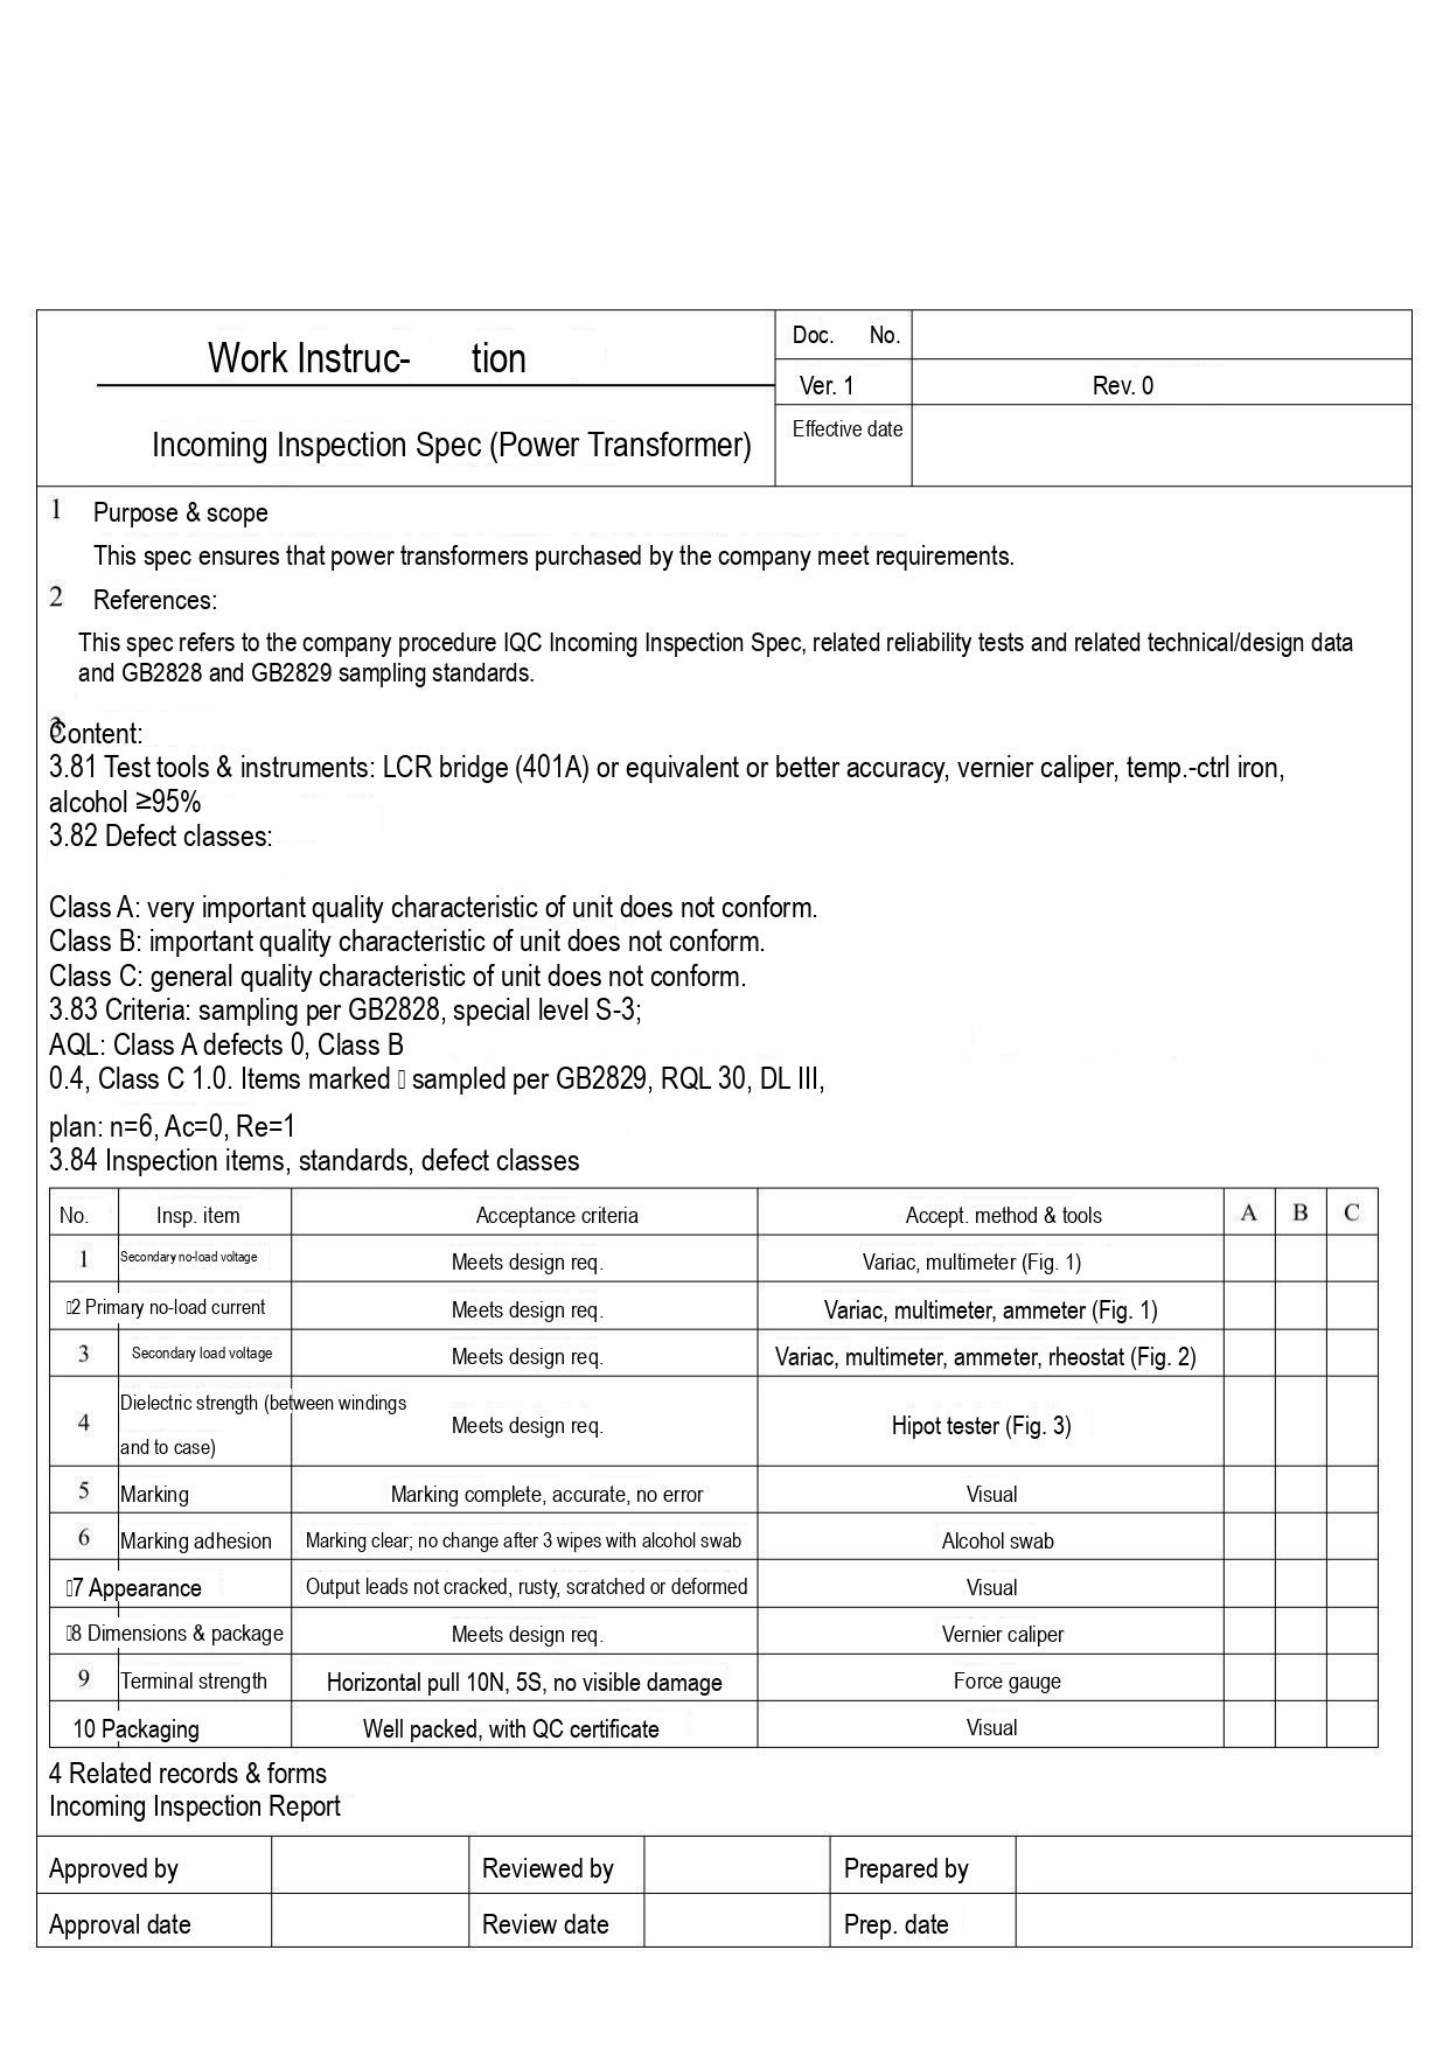| Work Instruc- tion<br>Incoming Inspection Spec (Power Transformer) | Doc. No. | |
|---|---|---|
| | Ver. 1 | Rev. 0 |
| | Effective date | |

1 Purpose & scope

This spec ensures that power transformers purchased by the company meet requirements.

2 References:

This spec refers to the company procedure IQC Incoming Inspection Spec, related reliability tests and related technical/design data and GB2828 and GB2829 sampling standards.

3 Content:
3.81 Test tools & instruments: LCR bridge (401A) or equivalent or better accuracy, vernier caliper, temp.-ctrl iron, alcohol ≥95%
3.82 Defect classes:

Class A: very important quality characteristic of unit does not conform.
Class B: important quality characteristic of unit does not conform.
Class C: general quality characteristic of unit does not conform.
3.83 Criteria: sampling per GB2828, special level S-3;
AQL: Class A defects 0, Class B
0.4, Class C 1.0. Items marked ▯ sampled per GB2829, RQL 30, DL III,

plan: n=6, Ac=0, Re=1
3.84 Inspection items, standards, defect classes

| No. | Insp. item | Acceptance criteria | Accept. method & tools | A | B | C |
|---|---|---|---|---|---|---|
| 1 | Secondary no-load voltage | Meets design req. | Variac, multimeter (Fig. 1) | | | |
| ▯2 | Primary no-load current | Meets design req. | Variac, multimeter, ammeter (Fig. 1) | | | |
| 3 | Secondary load voltage | Meets design req. | Variac, multimeter, ammeter, rheostat (Fig. 2) | | | |
| 4 | Dielectric strength (between windings and to case) | Meets design req. | Hipot tester (Fig. 3) | | | |
| 5 | Marking | Marking complete, accurate, no error | Visual | | | |
| 6 | Marking adhesion | Marking clear; no change after 3 wipes with alcohol swab | Alcohol swab | | | |
| ▯7 | Appearance | Output leads not cracked, rusty, scratched or deformed | Visual | | | |
| ▯8 | Dimensions & package | Meets design req. | Vernier caliper | | | |
| 9 | Terminal strength | Horizontal pull 10N, 5S, no visible damage | Force gauge | | | |
| 10 | Packaging | Well packed, with QC certificate | Visual | | | |

4 Related records & forms
Incoming Inspection Report

| Approved by | | Reviewed by | | Prepared by | |
|---|---|---|---|---|---|
| Approval date | | Review date | | Prep. date | |
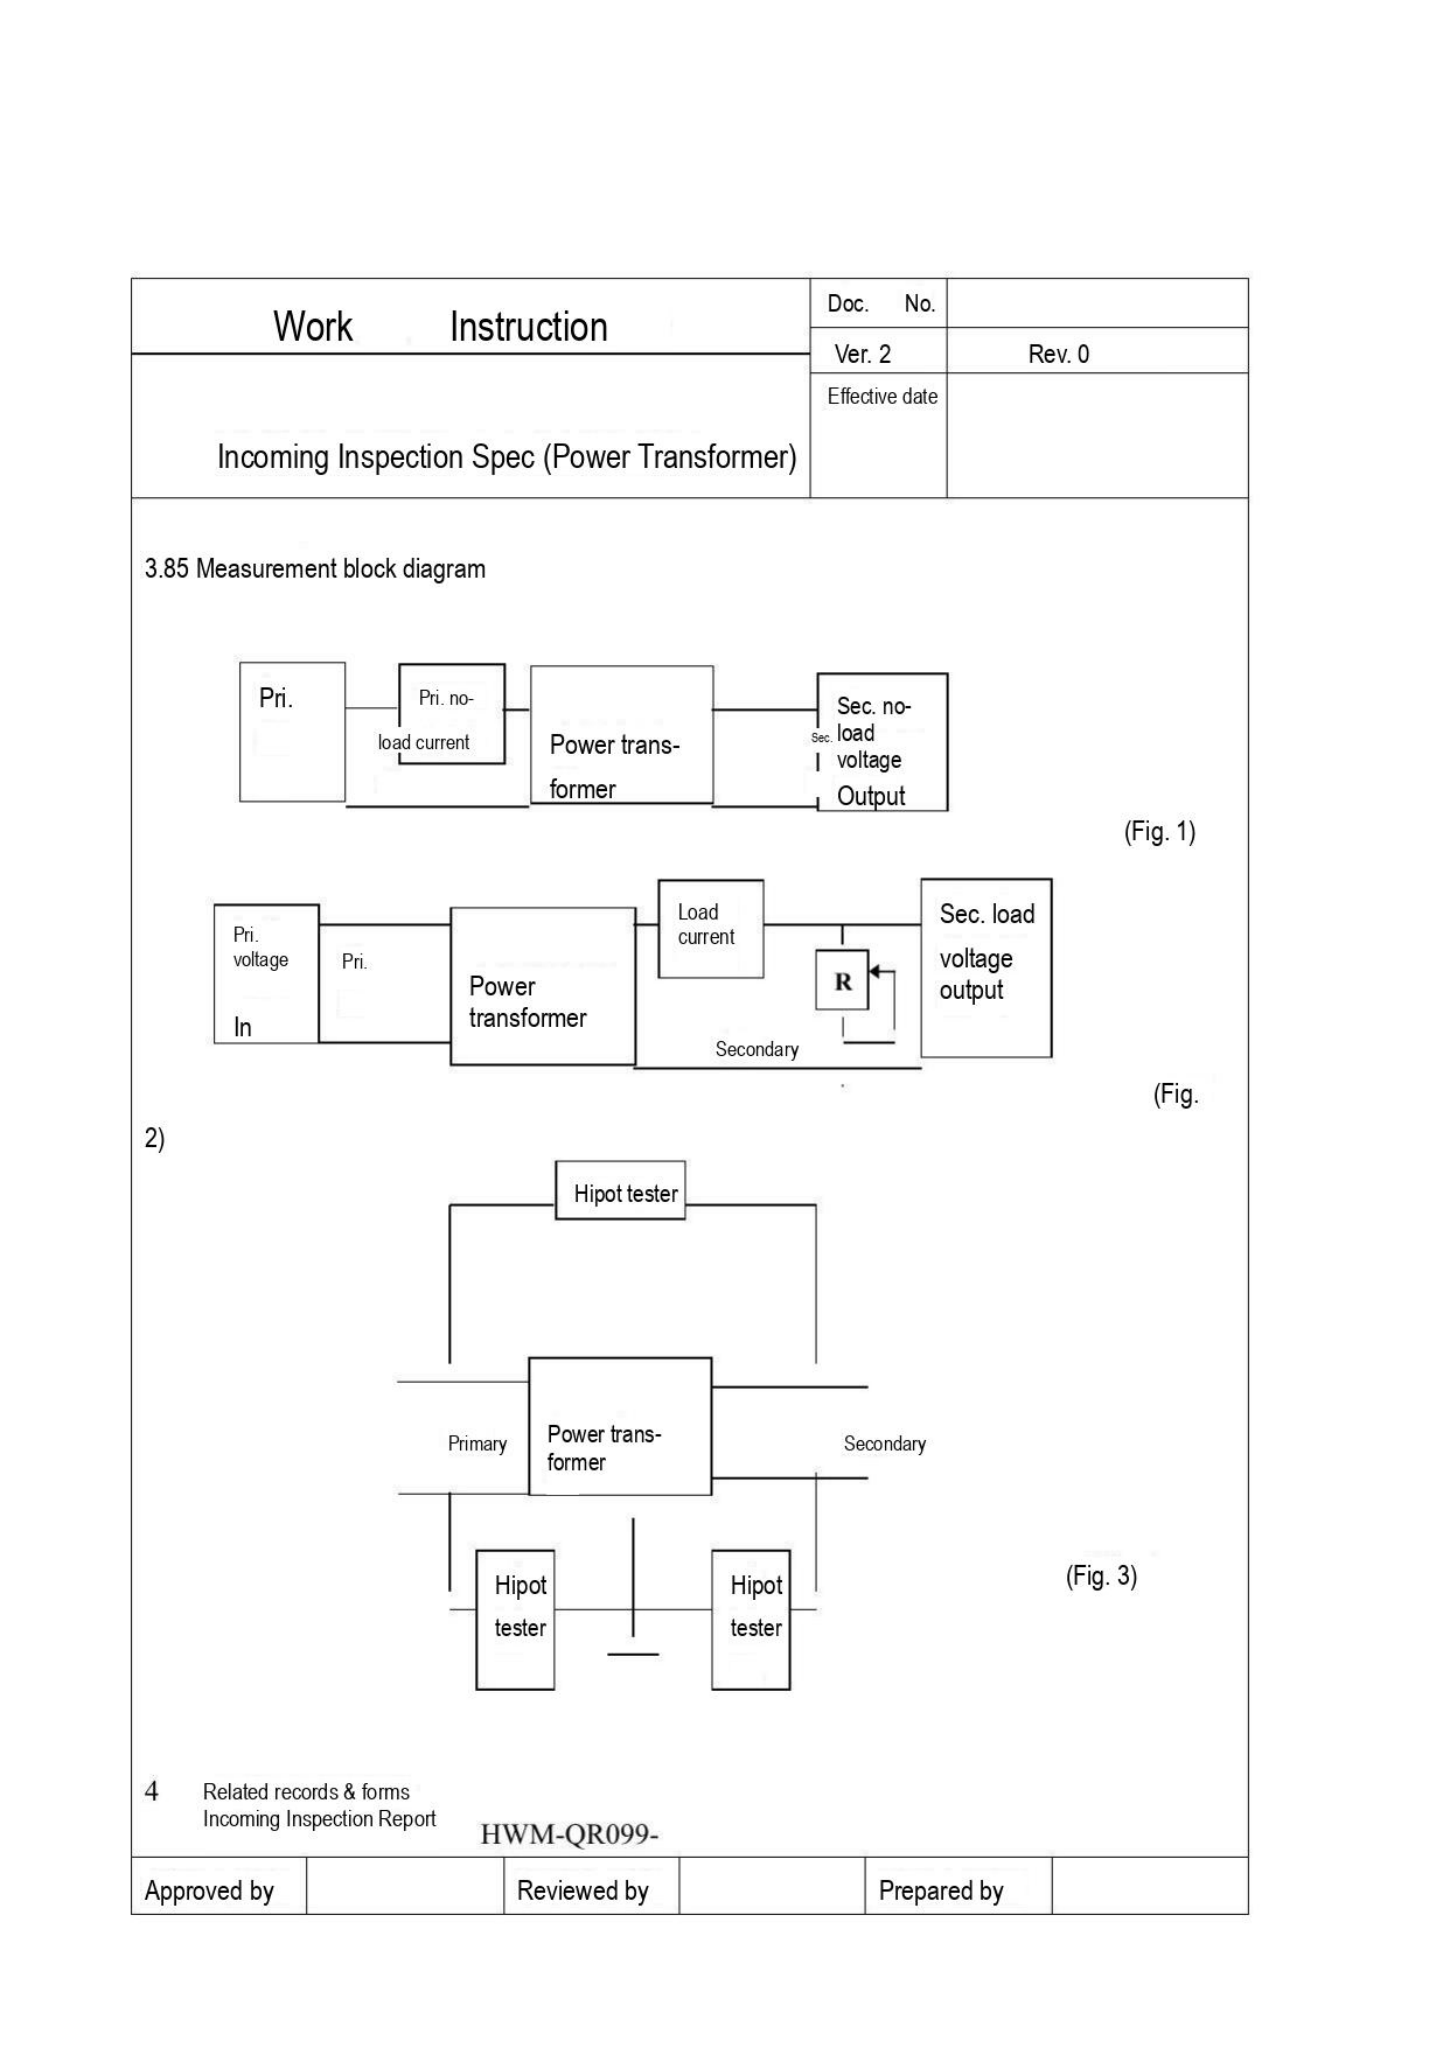| Work Instruction | Doc. No. | |
|---|---|---|
| | Ver. 2 | Rev. 0 |
| Incoming Inspection Spec (Power Transformer) | Effective date | |

3.85 Measurement block diagram

Pri.

Pri. no-load current

Power trans-former

Sec.

Sec. no-load voltage Output

(Fig. 1)

Pri. voltage In

Pri.

Power transformer

Load current

R

Secondary

Sec. load voltage output

(Fig. 2)

Hipot tester

Primary

Power trans-former

Secondary

Hipot tester

Hipot tester

(Fig. 3)

4 Related records & forms
Incoming Inspection Report HWM-QR099-

| Approved by | | Reviewed by | | Prepared by | |
|---|---|---|---|---|---|
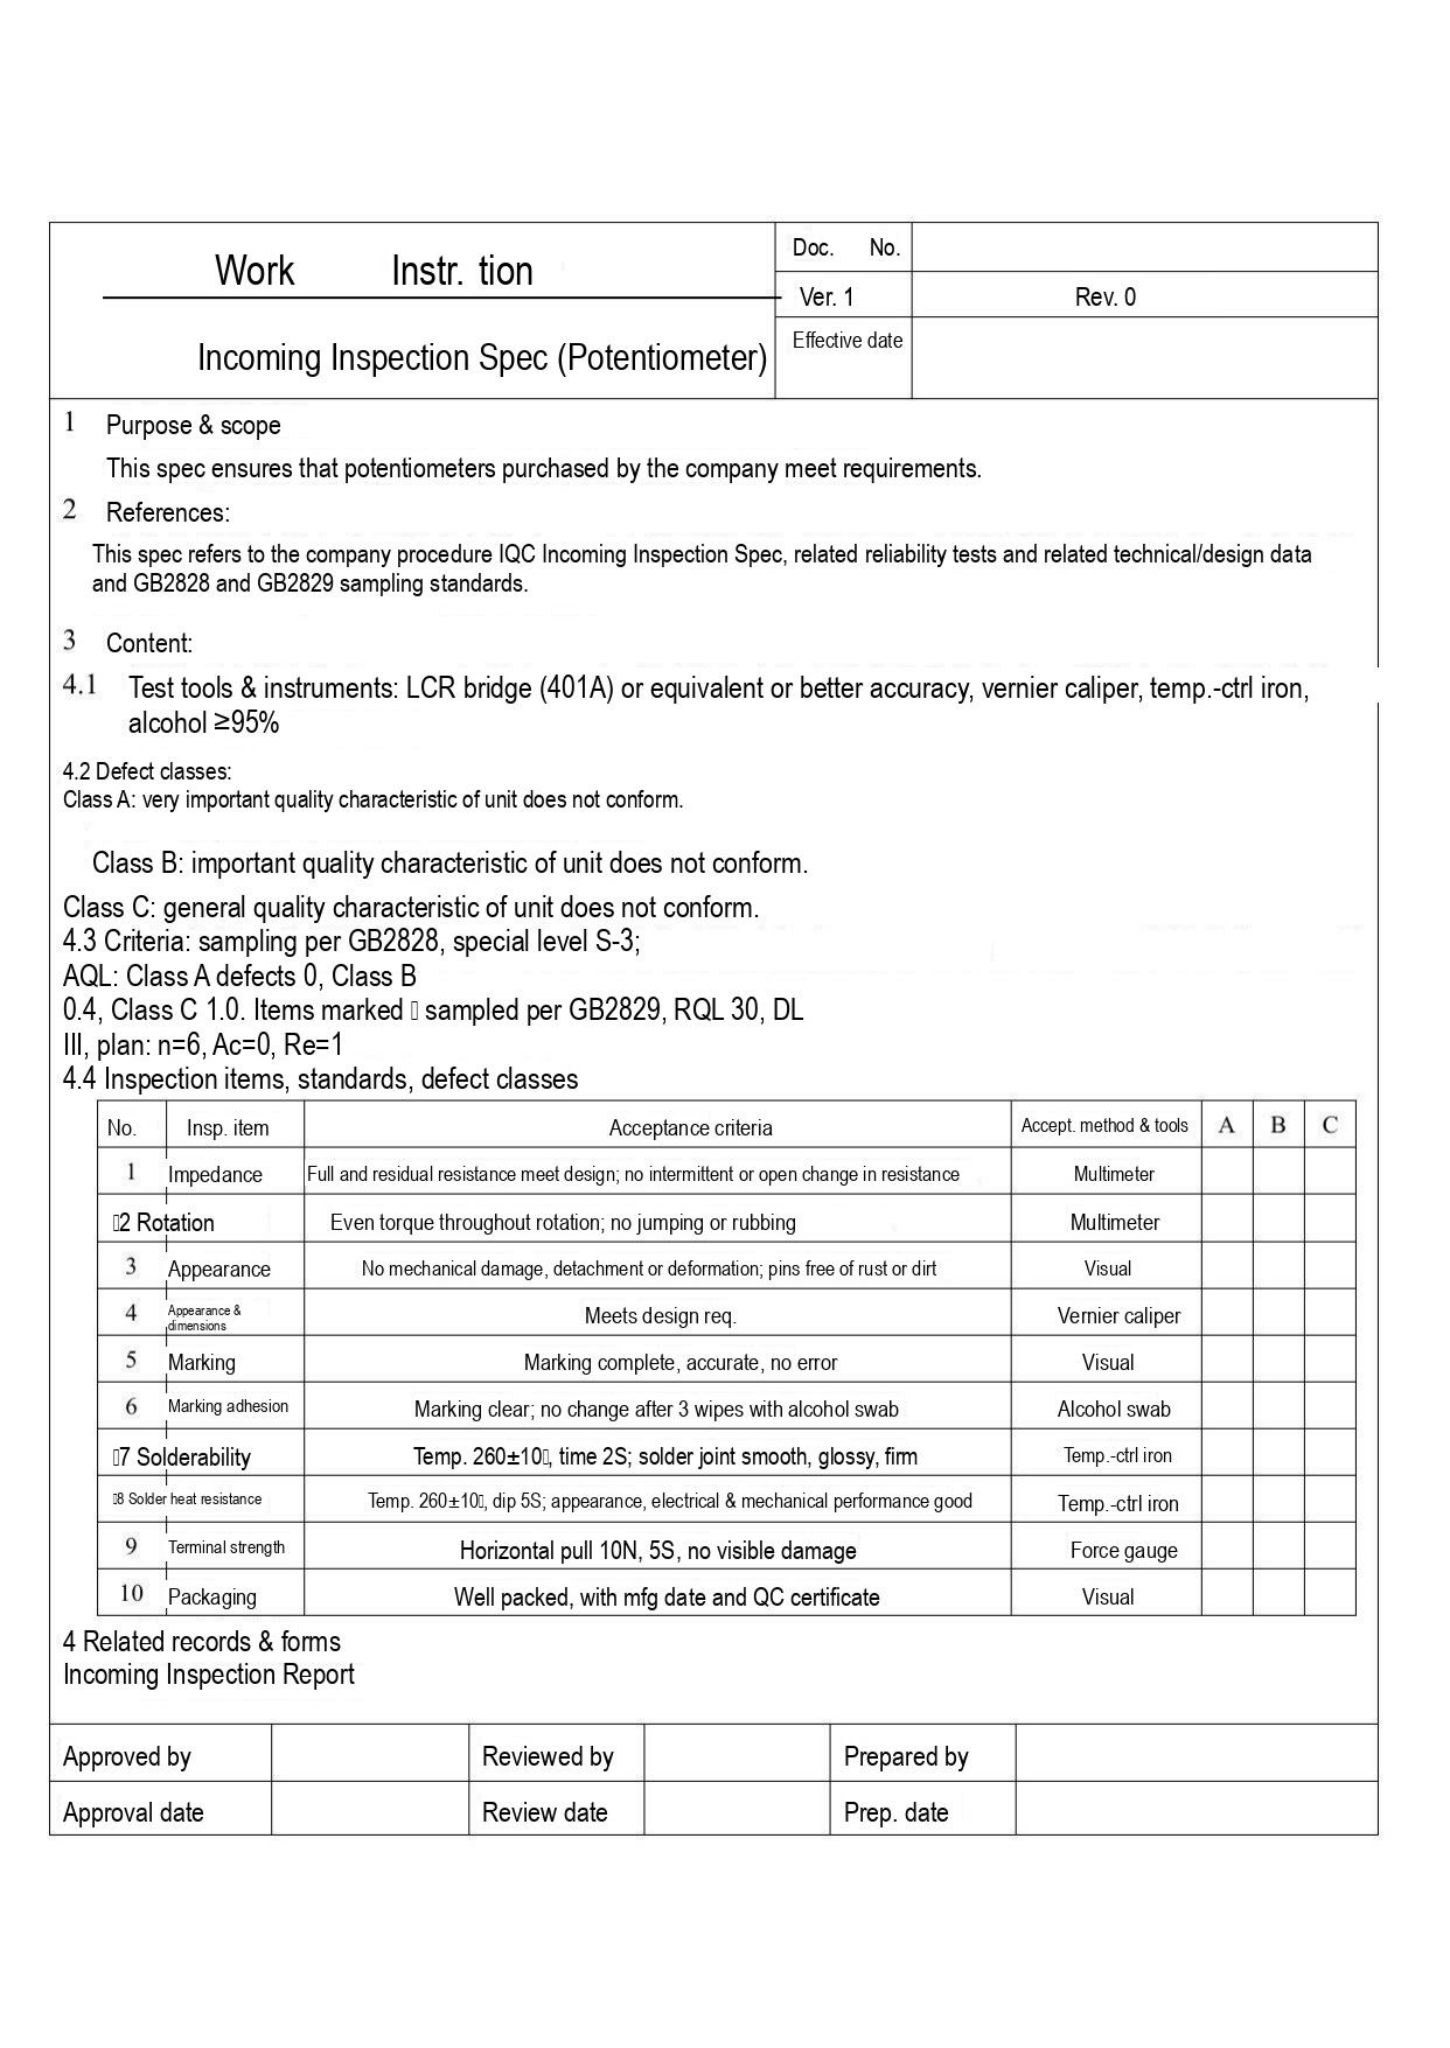| Work Instr. tion<br>Incoming Inspection Spec (Potentiometer) | Doc. No. | |
|---|---|---|
| | Ver. 1 | Rev. 0 |
| | Effective date | |

1 Purpose & scope

This spec ensures that potentiometers purchased by the company meet requirements.

2 References:

This spec refers to the company procedure IQC Incoming Inspection Spec, related reliability tests and related technical/design data and GB2828 and GB2829 sampling standards.

3 Content:

4.1 Test tools & instruments: LCR bridge (401A) or equivalent or better accuracy, vernier caliper, temp.-ctrl iron, alcohol ≥95%

4.2 Defect classes:
Class A: very important quality characteristic of unit does not conform.

Class B: important quality characteristic of unit does not conform.

Class C: general quality characteristic of unit does not conform.
4.3 Criteria: sampling per GB2828, special level S-3;
AQL: Class A defects 0, Class B
0.4, Class C 1.0. Items marked sampled per GB2829, RQL 30, DL
III, plan: n=6, Ac=0, Re=1
4.4 Inspection items, standards, defect classes

| No. | Insp. item | Acceptance criteria | Accept. method & tools | A | B | C |
|---|---|---|---|---|---|---|
| 1 | Impedance | Full and residual resistance meet design; no intermittent or open change in resistance | Multimeter | | | |
| 2 | Rotation | Even torque throughout rotation; no jumping or rubbing | Multimeter | | | |
| 3 | Appearance | No mechanical damage, detachment or deformation; pins free of rust or dirt | Visual | | | |
| 4 | Appearance & dimensions | Meets design req. | Vernier caliper | | | |
| 5 | Marking | Marking complete, accurate, no error | Visual | | | |
| 6 | Marking adhesion | Marking clear; no change after 3 wipes with alcohol swab | Alcohol swab | | | |
| 7 | Solderability | Temp. 260±10, time 2S; solder joint smooth, glossy, firm | Temp.-ctrl iron | | | |
| 8 | Solder heat resistance | Temp. 260±10, dip 5S; appearance, electrical & mechanical performance good | Temp.-ctrl iron | | | |
| 9 | Terminal strength | Horizontal pull 10N, 5S, no visible damage | Force gauge | | | |
| 10 | Packaging | Well packed, with mfg date and QC certificate | Visual | | | |

4 Related records & forms
Incoming Inspection Report

| Approved by | | Reviewed by | | Prepared by | |
|---|---|---|---|---|---|
| Approval date | | Review date | | Prep. date | |
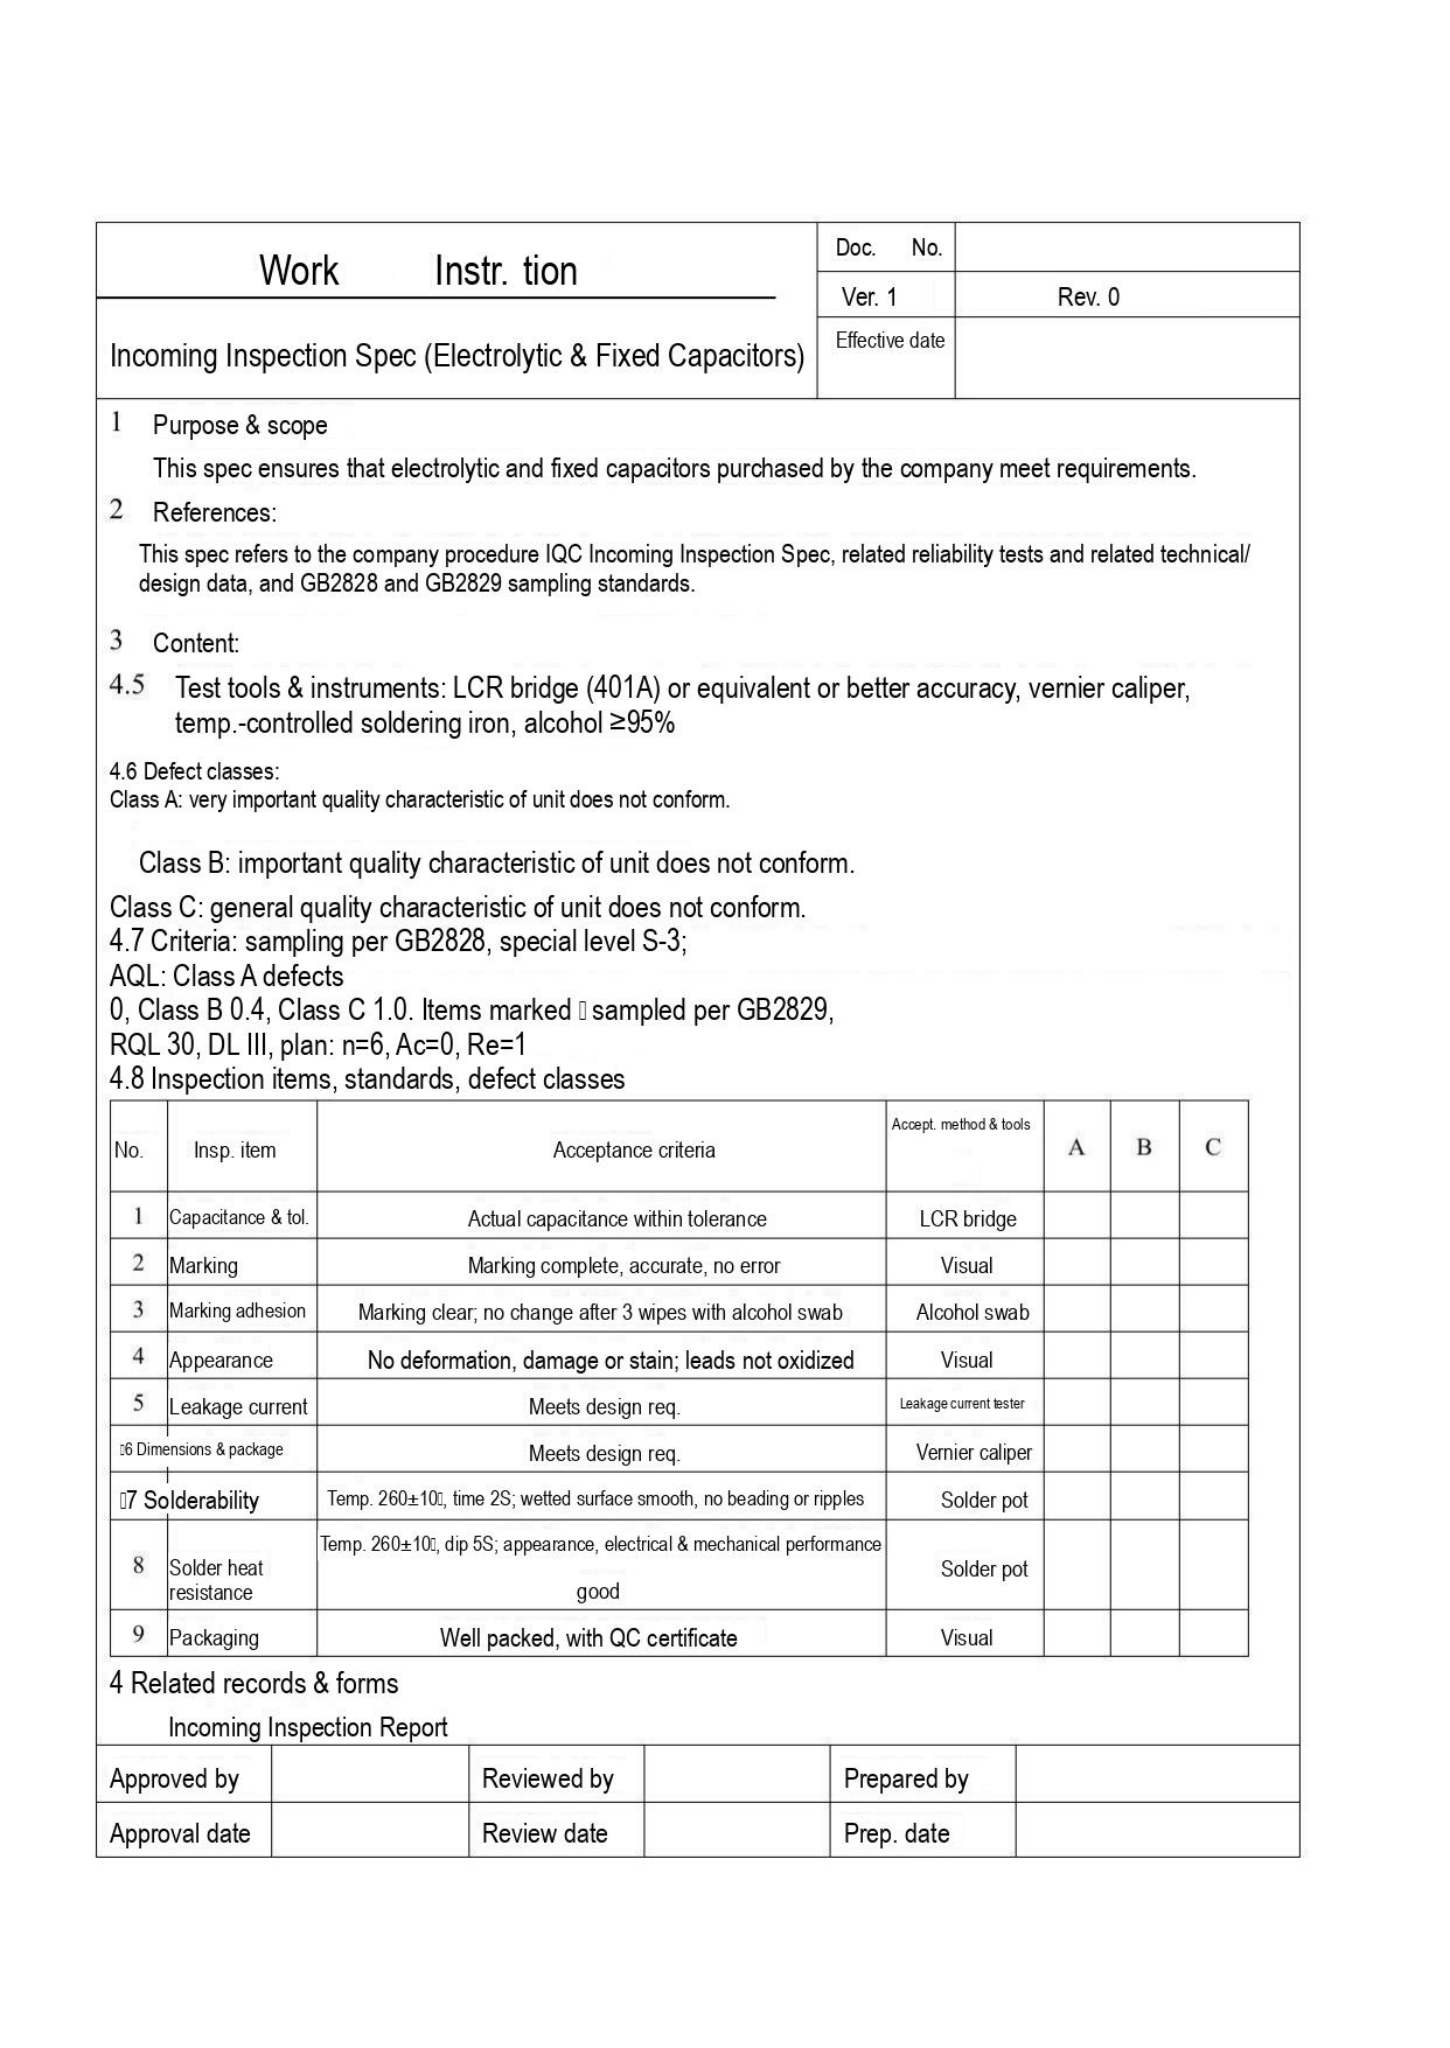| Work Instr. tion | Doc. No. | |
|---|---|---|
| | Ver. 1 | Rev. 0 |
| Incoming Inspection Spec (Electrolytic & Fixed Capacitors) | Effective date | |

1 Purpose & scope

This spec ensures that electrolytic and fixed capacitors purchased by the company meet requirements.

2 References:

This spec refers to the company procedure IQC Incoming Inspection Spec, related reliability tests and related technical/ design data, and GB2828 and GB2829 sampling standards.

3 Content:

4.5 Test tools & instruments: LCR bridge (401A) or equivalent or better accuracy, vernier caliper, temp.-controlled soldering iron, alcohol ≥95%

4.6 Defect classes:
Class A: very important quality characteristic of unit does not conform.

Class B: important quality characteristic of unit does not conform.

Class C: general quality characteristic of unit does not conform.
4.7 Criteria: sampling per GB2828, special level S-3;
AQL: Class A defects
0, Class B 0.4, Class C 1.0. Items marked sampled per GB2829,
RQL 30, DL III, plan: n=6, Ac=0, Re=1
4.8 Inspection items, standards, defect classes

| No. | Insp. item | Acceptance criteria | Accept. method & tools | A | B | C |
|---|---|---|---|---|---|---|
| 1 | Capacitance & tol. | Actual capacitance within tolerance | LCR bridge | | | |
| 2 | Marking | Marking complete, accurate, no error | Visual | | | |
| 3 | Marking adhesion | Marking clear; no change after 3 wipes with alcohol swab | Alcohol swab | | | |
| 4 | Appearance | No deformation, damage or stain; leads not oxidized | Visual | | | |
| 5 | Leakage current | Meets design req. | Leakage current tester | | | |
| 6 | Dimensions & package | Meets design req. | Vernier caliper | | | |
| 7 | Solderability | Temp. 260±10, time 2S; wetted surface smooth, no beading or ripples | Solder pot | | | |
| 8 | Solder heat resistance | Temp. 260±10, dip 5S; appearance, electrical & mechanical performance good | Solder pot | | | |
| 9 | Packaging | Well packed, with QC certificate | Visual | | | |

4 Related records & forms

Incoming Inspection Report

| Approved by | | Reviewed by | | Prepared by | |
|---|---|---|---|---|---|
| Approval date | | Review date | | Prep. date | |
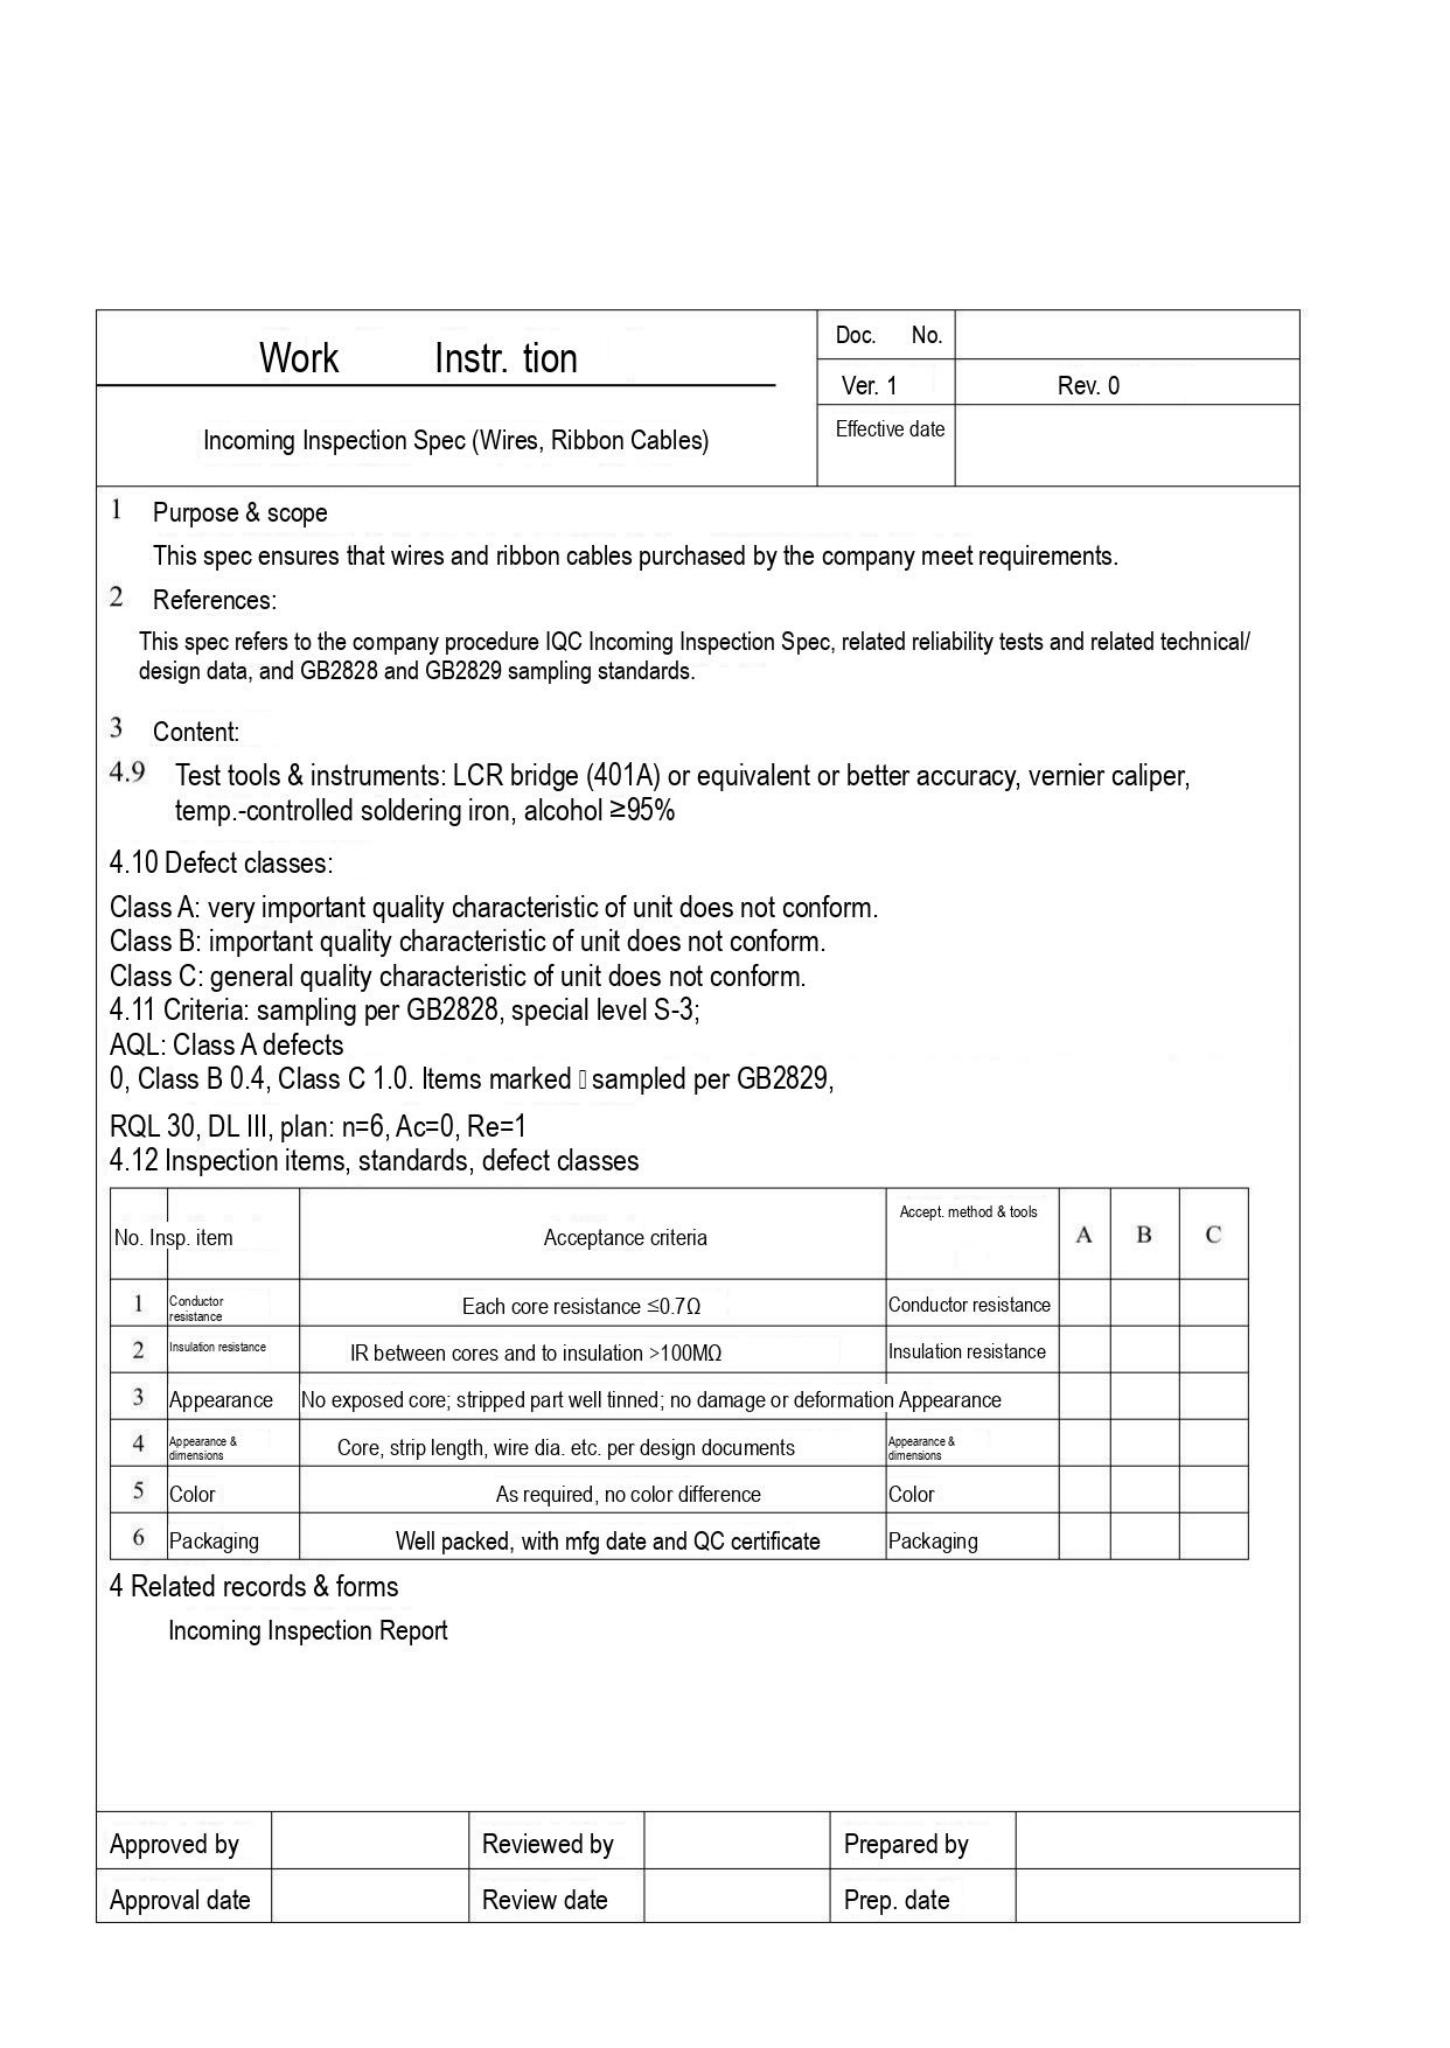| Work Instr. tion | Doc. No. | |
|---|---|---|
| | Ver. 1 | Rev. 0 |
| Incoming Inspection Spec (Wires, Ribbon Cables) | Effective date | |

1 Purpose & scope

This spec ensures that wires and ribbon cables purchased by the company meet requirements.

2 References:

This spec refers to the company procedure IQC Incoming Inspection Spec, related reliability tests and related technical/ design data, and GB2828 and GB2829 sampling standards.

3 Content:

4.9 Test tools & instruments: LCR bridge (401A) or equivalent or better accuracy, vernier caliper, temp.-controlled soldering iron, alcohol ≥95%

4.10 Defect classes:

Class A: very important quality characteristic of unit does not conform.
Class B: important quality characteristic of unit does not conform.
Class C: general quality characteristic of unit does not conform.
4.11 Criteria: sampling per GB2828, special level S-3;
AQL: Class A defects
0, Class B 0.4, Class C 1.0. Items marked sampled per GB2829,

RQL 30, DL III, plan: n=6, Ac=0, Re=1
4.12 Inspection items, standards, defect classes

| No. | Insp. item | Acceptance criteria | Accept. method & tools | A | B | C |
|---|---|---|---|---|---|---|
| 1 | Conductor resistance | Each core resistance ≤0.7Ω | Conductor resistance | | | |
| 2 | Insulation resistance | IR between cores and to insulation >100MΩ | Insulation resistance | | | |
| 3 | Appearance | No exposed core; stripped part well tinned; no damage or deformation | Appearance | | | |
| 4 | Appearance & dimensions | Core, strip length, wire dia. etc. per design documents | Appearance & dimensions | | | |
| 5 | Color | As required, no color difference | Color | | | |
| 6 | Packaging | Well packed, with mfg date and QC certificate | Packaging | | | |

4 Related records & forms

Incoming Inspection Report

| Approved by | | Reviewed by | | Prepared by | |
|---|---|---|---|---|---|
| Approval date | | Review date | | Prep. date | |
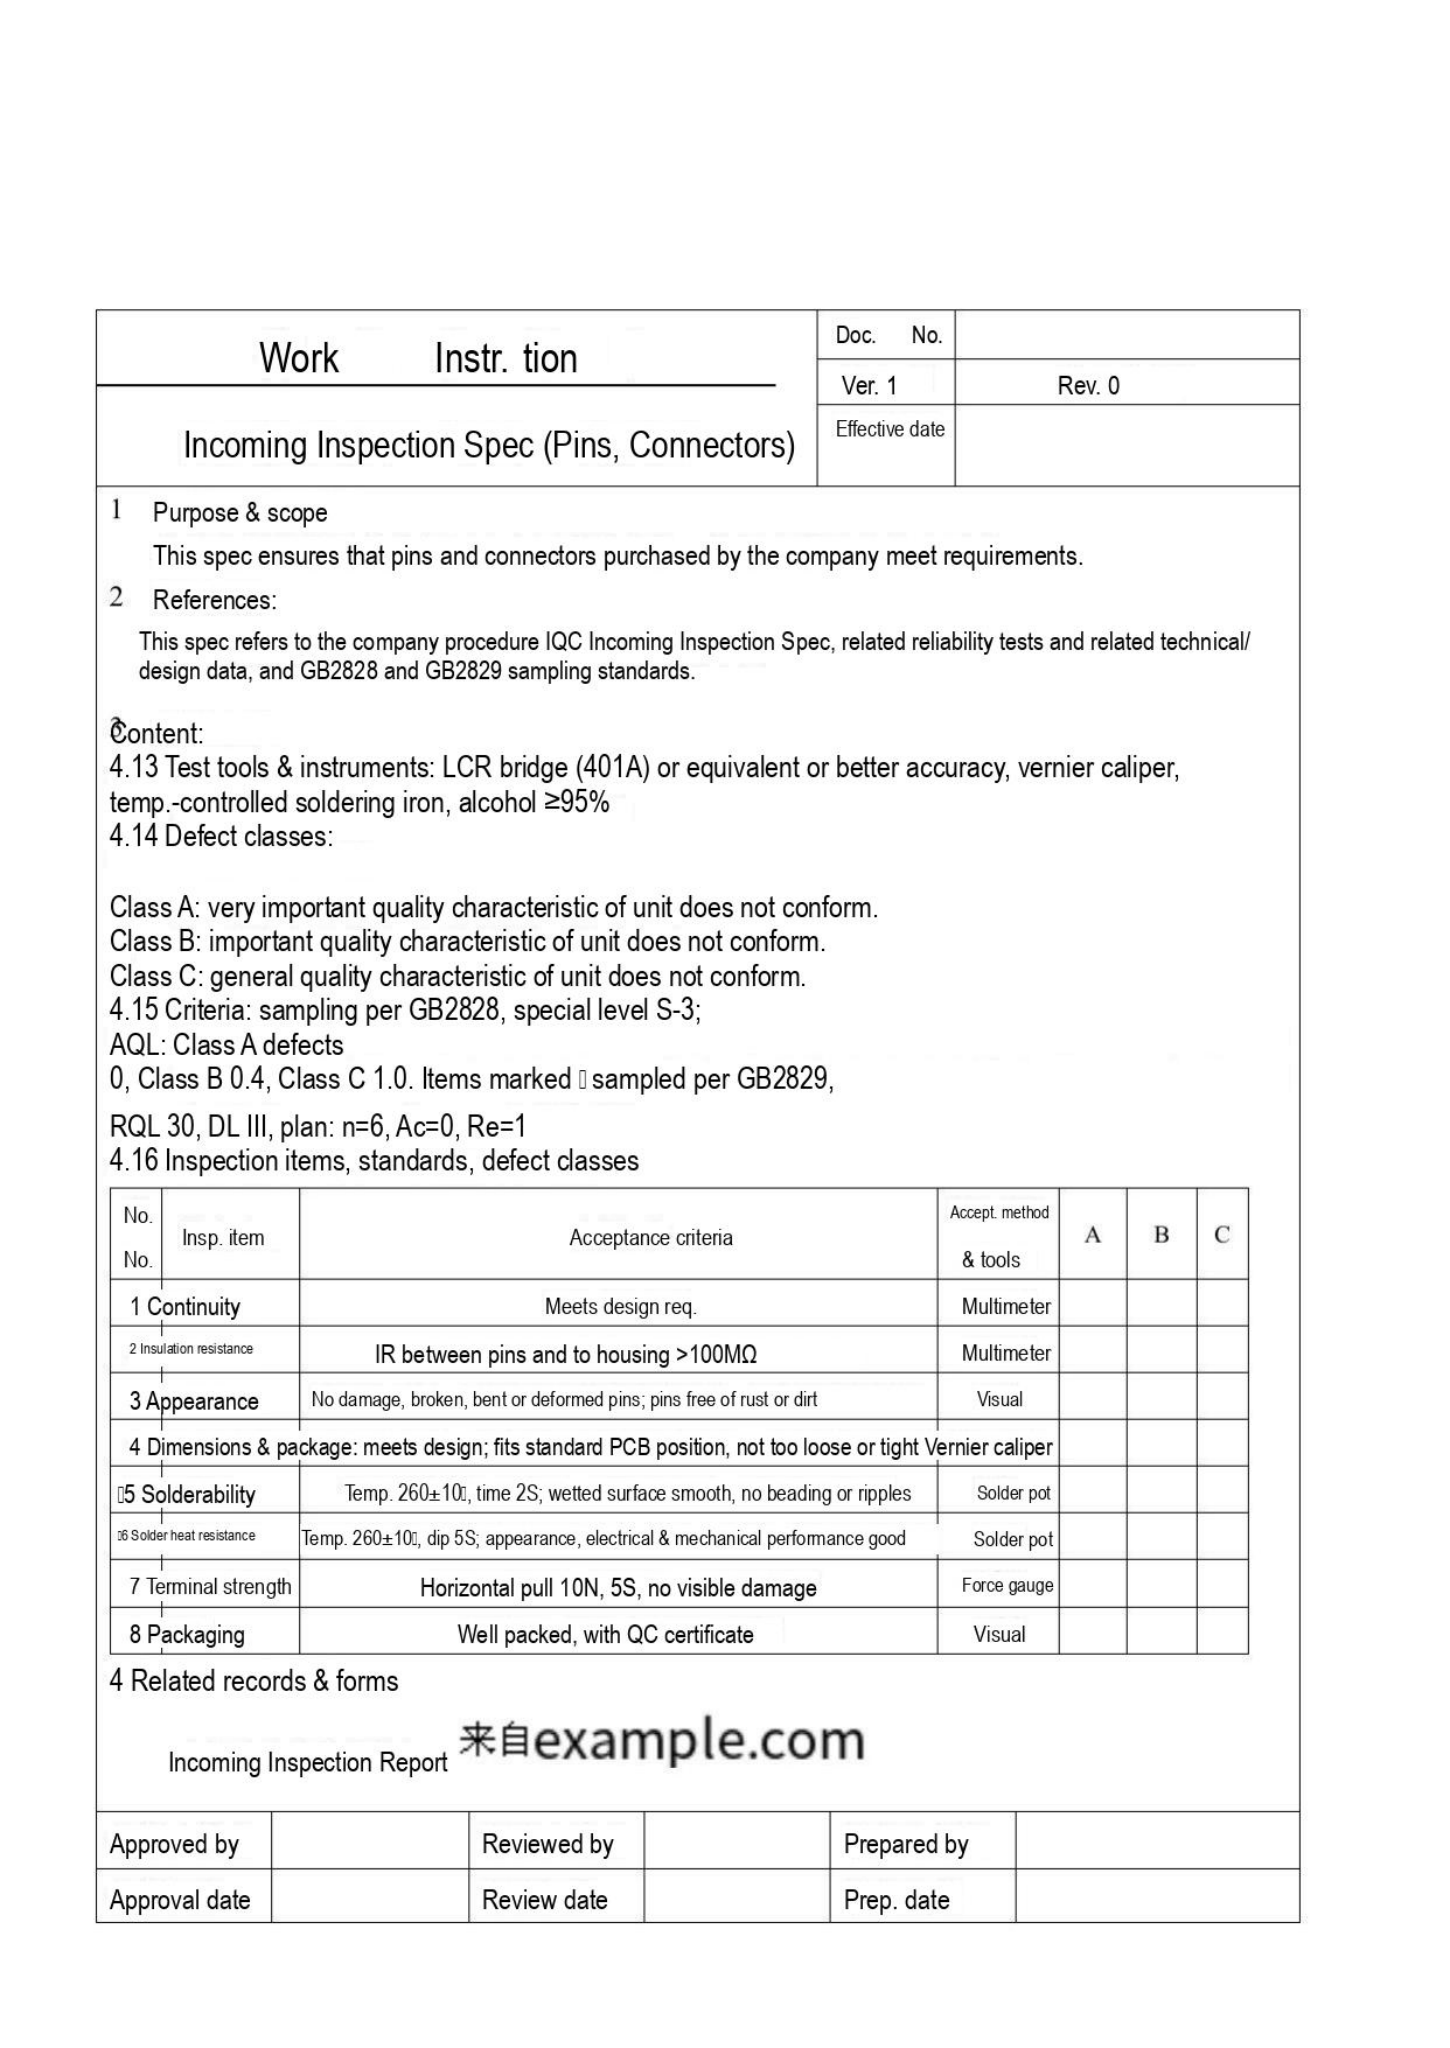| Work Instr. tion | Doc. No. | |
|---|---|---|
| | Ver. 1 | Rev. 0 |
| Incoming Inspection Spec (Pins, Connectors) | Effective date | |

1 Purpose & scope

This spec ensures that pins and connectors purchased by the company meet requirements.

2 References:

This spec refers to the company procedure IQC Incoming Inspection Spec, related reliability tests and related technical/ design data, and GB2828 and GB2829 sampling standards.

3 Content:
4.13 Test tools & instruments: LCR bridge (401A) or equivalent or better accuracy, vernier caliper, temp.-controlled soldering iron, alcohol ≥95%
4.14 Defect classes:

Class A: very important quality characteristic of unit does not conform.
Class B: important quality characteristic of unit does not conform.
Class C: general quality characteristic of unit does not conform.
4.15 Criteria: sampling per GB2828, special level S-3;
AQL: Class A defects
0, Class B 0.4, Class C 1.0. Items marked sampled per GB2829,

RQL 30, DL III, plan: n=6, Ac=0, Re=1
4.16 Inspection items, standards, defect classes

| No. No. | Insp. item | Acceptance criteria | Accept. method & tools | A | B | C |
|---|---|---|---|---|---|---|
| 1 | Continuity | Meets design req. | Multimeter | | | |
| 2 | Insulation resistance | IR between pins and to housing >100MΩ | Multimeter | | | |
| 3 | Appearance | No damage, broken, bent or deformed pins; pins free of rust or dirt | Visual | | | |
| 4 | Dimensions & package: | meets design; fits standard PCB position, not too loose or tight | Vernier caliper | | | |
| 5 | Solderability | Temp. 260±10, time 2S; wetted surface smooth, no beading or ripples | Solder pot | | | |
| 6 | Solder heat resistance | Temp. 260±10, dip 5S; appearance, electrical & mechanical performance good | Solder pot | | | |
| 7 | Terminal strength | Horizontal pull 10N, 5S, no visible damage | Force gauge | | | |
| 8 | Packaging | Well packed, with QC certificate | Visual | | | |

4 Related records & forms

Incoming Inspection Report 来自example.com

| Approved by | | Reviewed by | | Prepared by | |
|---|---|---|---|---|---|
| Approval date | | Review date | | Prep. date | |